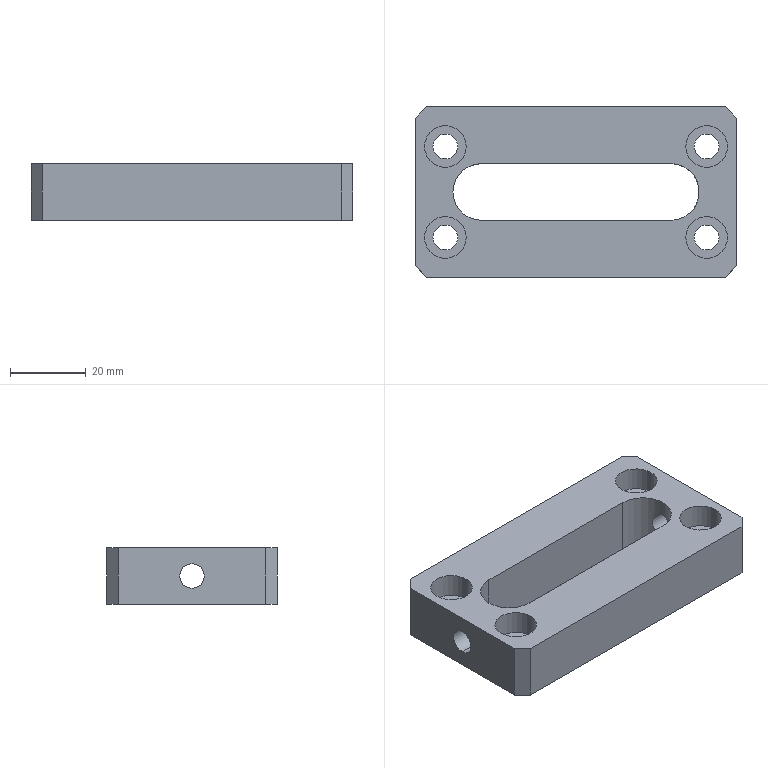Part | SolidWorks | features Chamfer 1, Extrusion 1, HoleWzd 1, ICE 1 | 1 solid | 39 faces | box 85 x 45 x 15 mm | volume 38919 mm3 | cylinder 23 | plane 16 | commonest cylinder face diameters 6.6 x8 11 x8 6.5 x4 15 x3
STEP:
#1=CARTESIAN_POINT('',(-32.5,0.,10.75));
#2=VERTEX_POINT('',#1);
#3=CARTESIAN_POINT('',(-32.5,0.,4.25));
#4=VERTEX_POINT('',#3);
#5=CARTESIAN_POINT('',(-32.5,0.,10.75));
#6=CARTESIAN_POINT('',(-32.5,-0.2176,10.75));
#7=CARTESIAN_POINT('',(-32.491,-0.4312,10.728));
#8=CARTESIAN_POINT('',(-32.455,-0.8504,10.644));
#9=CARTESIAN_POINT('',(-32.428,-1.058,10.58));
#10=CARTESIAN_POINT('',(-32.361,-1.451,10.416));
#11=CARTESIAN_POINT('',(-32.321,-1.637,10.316));
#12=CARTESIAN_POINT('',(-32.234,-1.988,10.08));
#13=CARTESIAN_POINT('',(-32.186,-2.152,9.944));
#14=CARTESIAN_POINT('',(-32.091,-2.448,9.648));
#15=CARTESIAN_POINT('',(-32.043,-2.582,9.485));
#16=CARTESIAN_POINT('',(-31.952,-2.818,9.133));
#17=CARTESIAN_POINT('',(-31.91,-2.917,8.948));
#18=CARTESIAN_POINT('',(-31.839,-3.08,8.558));
#19=CARTESIAN_POINT('',(-31.809,-3.144,8.351));
#20=CARTESIAN_POINT('',(-31.77,-3.229,7.93));
#21=CARTESIAN_POINT('',(-31.759,-3.25,7.717));
#22=CARTESIAN_POINT('',(-31.759,-3.25,7.287));
#23=CARTESIAN_POINT('',(-31.77,-3.228,7.069));
#24=CARTESIAN_POINT('',(-31.809,-3.144,6.65));
#25=CARTESIAN_POINT('',(-31.838,-3.081,6.445));
#26=CARTESIAN_POINT('',(-31.91,-2.916,6.05));
#27=CARTESIAN_POINT('',(-31.952,-2.816,5.864));
#28=CARTESIAN_POINT('',(-32.043,-2.581,5.514));
#29=CARTESIAN_POINT('',(-32.092,-2.446,5.349));
#30=CARTESIAN_POINT('',(-32.187,-2.149,5.053));
#31=CARTESIAN_POINT('',(-32.234,-1.987,4.92));
#32=CARTESIAN_POINT('',(-32.322,-1.636,4.684));
#33=CARTESIAN_POINT('',(-32.362,-1.447,4.582));
#34=CARTESIAN_POINT('',(-32.428,-1.057,4.419));
#35=CARTESIAN_POINT('',(-32.454,-0.8534,4.357));
#36=CARTESIAN_POINT('',(-32.491,-0.4282,4.271));
#37=CARTESIAN_POINT('',(-32.5,-0.2144,4.25));
#38=CARTESIAN_POINT('',(-32.5,0.,4.25));
#39=B_SPLINE_CURVE_WITH_KNOTS('',3,(#5,#6,#7,#8,#9,#10,#11,#12,#13,#14,#15,#16,#17,#18,#19,#20,#21,#22,#23,#24,#25,#26,#27,#28,#29,#30,#31,#32,#33,#34,#35,#36,#37,#38),.UNSPECIFIED.,.F.,.F.,(4,2,2,2,2,2,2,2,2,2,2,2,2,2,2,2,4),(0.,0.0006431,0.001286,0.001929,0.002573,0.003216,0.003859,0.004502,0.005145,0.005788,0.006431,0.007074,0.007718,0.008361,0.009004,0.009647,0.01029),.UNSPECIFIED.);
#40=EDGE_CURVE('',#2,#4,#39,.T.);
#41=ORIENTED_EDGE('',*,*,#40,.T.);
#42=CARTESIAN_POINT('',(-42.5,0.,4.25));
#43=VERTEX_POINT('',#42);
#44=CARTESIAN_POINT('',(119.5,0.,4.25));
#45=DIRECTION('',(-1.,0.,0.));
#46=VECTOR('',#45,1000.);
#47=LINE('',#44,#46);
#48=EDGE_CURVE('',#4,#43,#47,.T.);
#49=ORIENTED_EDGE('',*,*,#48,.T.);
#50=CARTESIAN_POINT('',(-42.5,0.,10.75));
#51=VERTEX_POINT('',#50);
#52=CARTESIAN_POINT('',(-42.5,0.,7.5));
#53=DIRECTION('',(-1.,0.,0.));
#54=DIRECTION('',(0.,0.,1.));
#55=AXIS2_PLACEMENT_3D('',#52,#53,#54);
#56=CIRCLE('',#55,3.25);
#57=EDGE_CURVE('',#43,#51,#56,.T.);
#58=ORIENTED_EDGE('',*,*,#57,.T.);
#59=CARTESIAN_POINT('',(119.5,0.,10.75));
#60=DIRECTION('',(-1.,0.,0.));
#61=VECTOR('',#60,1000.);
#62=LINE('',#59,#61);
#63=EDGE_CURVE('',#2,#51,#62,.T.);
#64=ORIENTED_EDGE('',*,*,#63,.F.);
#65=EDGE_LOOP('',(#41,#49,#58,#64));
#66=FACE_OUTER_BOUND('',#65,.T.);
#67=CARTESIAN_POINT('',(119.5,0.,7.5));
#68=DIRECTION('',(-1.,0.,0.));
#69=DIRECTION('',(0.,0.,1.));
#70=AXIS2_PLACEMENT_3D('',#67,#68,#69);
#71=CYLINDRICAL_SURFACE('',#70,3.25);
#72=ADVANCED_FACE('',(#66),#71,.F.);
#73=CARTESIAN_POINT('',(42.5,0.,4.25));
#74=VERTEX_POINT('',#73);
#75=CARTESIAN_POINT('',(42.5,0.,10.75));
#76=VERTEX_POINT('',#75);
#77=CARTESIAN_POINT('',(42.5,0.,7.5));
#78=DIRECTION('',(-1.,0.,0.));
#79=DIRECTION('',(0.,0.,1.));
#80=AXIS2_PLACEMENT_3D('',#77,#78,#79);
#81=CIRCLE('',#80,3.25);
#82=EDGE_CURVE('',#74,#76,#81,.T.);
#83=ORIENTED_EDGE('',*,*,#82,.F.);
#84=CARTESIAN_POINT('',(32.5,0.,4.25));
#85=VERTEX_POINT('',#84);
#86=CARTESIAN_POINT('',(119.5,0.,4.25));
#87=DIRECTION('',(-1.,0.,0.));
#88=VECTOR('',#87,1000.);
#89=LINE('',#86,#88);
#90=EDGE_CURVE('',#74,#85,#89,.T.);
#91=ORIENTED_EDGE('',*,*,#90,.T.);
#92=CARTESIAN_POINT('',(32.5,0.,10.75));
#93=VERTEX_POINT('',#92);
#94=CARTESIAN_POINT('',(32.5,0.,4.25));
#95=CARTESIAN_POINT('',(32.5,-0.2142,4.25));
#96=CARTESIAN_POINT('',(32.491,-0.4319,4.272));
#97=CARTESIAN_POINT('',(32.454,-0.8529,4.357));
#98=CARTESIAN_POINT('',(32.428,-1.056,4.419));
#99=CARTESIAN_POINT('',(32.361,-1.45,4.584));
#100=CARTESIAN_POINT('',(32.321,-1.639,4.686));
#101=CARTESIAN_POINT('',(32.234,-1.988,4.92));
#102=CARTESIAN_POINT('',(32.187,-2.151,5.055));
#103=CARTESIAN_POINT('',(32.091,-2.449,5.353));
#104=CARTESIAN_POINT('',(32.043,-2.582,5.515));
#105=CARTESIAN_POINT('',(31.952,-2.816,5.864));
#106=CARTESIAN_POINT('',(31.91,-2.918,6.053));
#107=CARTESIAN_POINT('',(31.839,-3.081,6.444));
#108=CARTESIAN_POINT('',(31.81,-3.143,6.646));
#109=CARTESIAN_POINT('',(31.77,-3.228,7.066));
#110=CARTESIAN_POINT('',(31.759,-3.25,7.284));
#111=CARTESIAN_POINT('',(31.759,-3.25,7.713));
#112=CARTESIAN_POINT('',(31.769,-3.229,7.927));
#113=CARTESIAN_POINT('',(31.809,-3.144,8.351));
#114=CARTESIAN_POINT('',(31.838,-3.081,8.555));
#115=CARTESIAN_POINT('',(31.91,-2.918,8.947));
#116=CARTESIAN_POINT('',(31.952,-2.816,9.136));
#117=CARTESIAN_POINT('',(32.043,-2.582,9.485));
#118=CARTESIAN_POINT('',(32.091,-2.449,9.647));
#119=CARTESIAN_POINT('',(32.235,-2.001,10.095));
#120=CARTESIAN_POINT('',(32.327,-1.649,10.333));
#121=CARTESIAN_POINT('',(32.428,-1.056,10.581));
#122=CARTESIAN_POINT('',(32.454,-0.853,10.643));
#123=CARTESIAN_POINT('',(32.49,-0.4346,10.728));
#124=CARTESIAN_POINT('',(32.5,-0.2174,10.75));
#125=CARTESIAN_POINT('',(32.5,0.,10.75));
#126=B_SPLINE_CURVE_WITH_KNOTS('',3,(#94,#95,#96,#97,#98,#99,#100,#101,#102,#103,#104,#105,#106,#107,#108,#109,#110,#111,#112,#113,#114,#115,#116,#117,#118,#119,#120,#121,#122,#123,#124,#125),.UNSPECIFIED.,.F.,.F.,(4,2,2,2,2,2,2,2,2,2,2,2,2,2,2,4),(0.01029,0.01093,0.01158,0.01222,0.01286,0.0135,0.01415,0.01479,0.01543,0.01607,0.01672,0.01736,0.018,0.01929,0.01993,0.02057),.UNSPECIFIED.);
#127=EDGE_CURVE('',#85,#93,#126,.T.);
#128=ORIENTED_EDGE('',*,*,#127,.T.);
#129=CARTESIAN_POINT('',(119.5,0.,10.75));
#130=DIRECTION('',(-1.,0.,0.));
#131=VECTOR('',#130,1000.);
#132=LINE('',#129,#131);
#133=EDGE_CURVE('',#76,#93,#132,.T.);
#134=ORIENTED_EDGE('',*,*,#133,.F.);
#135=EDGE_LOOP('',(#83,#91,#128,#134));
#136=FACE_OUTER_BOUND('',#135,.T.);
#137=CARTESIAN_POINT('',(119.5,0.,7.5));
#138=DIRECTION('',(-1.,0.,0.));
#139=DIRECTION('',(0.,0.,1.));
#140=AXIS2_PLACEMENT_3D('',#137,#138,#139);
#141=CYLINDRICAL_SURFACE('',#140,3.25);
#142=ADVANCED_FACE('',(#136),#141,.F.);
#143=CARTESIAN_POINT('',(-40.,12.,8.6));
#144=VERTEX_POINT('',#143);
#145=CARTESIAN_POINT('',(-29.,12.,8.6));
#146=VERTEX_POINT('',#145);
#147=CARTESIAN_POINT('',(-34.5,12.,8.6));
#148=DIRECTION('',(0.,0.,1.));
#149=DIRECTION('',(1.,0.,0.));
#150=AXIS2_PLACEMENT_3D('',#147,#148,#149);
#151=CIRCLE('',#150,5.5);
#152=EDGE_CURVE('',#144,#146,#151,.T.);
#153=ORIENTED_EDGE('',*,*,#152,.F.);
#154=CARTESIAN_POINT('',(-40.,12.,15.));
#155=VERTEX_POINT('',#154);
#156=CARTESIAN_POINT('',(-40.,12.,15.));
#157=DIRECTION('',(0.,0.,1.));
#158=VECTOR('',#157,1000.);
#159=LINE('',#156,#158);
#160=EDGE_CURVE('',#144,#155,#159,.T.);
#161=ORIENTED_EDGE('',*,*,#160,.T.);
#162=CARTESIAN_POINT('',(-29.,12.,15.));
#163=VERTEX_POINT('',#162);
#164=CARTESIAN_POINT('',(-34.5,12.,15.));
#165=DIRECTION('',(0.,0.,1.));
#166=DIRECTION('',(1.,0.,0.));
#167=AXIS2_PLACEMENT_3D('',#164,#165,#166);
#168=CIRCLE('',#167,5.5);
#169=EDGE_CURVE('',#155,#163,#168,.T.);
#170=ORIENTED_EDGE('',*,*,#169,.T.);
#171=CARTESIAN_POINT('',(-29.,12.,15.));
#172=DIRECTION('',(0.,0.,1.));
#173=VECTOR('',#172,1000.);
#174=LINE('',#171,#173);
#175=EDGE_CURVE('',#146,#163,#174,.T.);
#176=ORIENTED_EDGE('',*,*,#175,.F.);
#177=EDGE_LOOP('',(#153,#161,#170,#176));
#178=FACE_OUTER_BOUND('',#177,.T.);
#179=CARTESIAN_POINT('',(-34.5,12.,15.));
#180=DIRECTION('',(0.,0.,1.));
#181=DIRECTION('',(1.,0.,0.));
#182=AXIS2_PLACEMENT_3D('',#179,#180,#181);
#183=CYLINDRICAL_SURFACE('',#182,5.5);
#184=ADVANCED_FACE('',(#178),#183,.F.);
#185=CARTESIAN_POINT('',(-37.8,12.,0.));
#186=VERTEX_POINT('',#185);
#187=CARTESIAN_POINT('',(-31.2,12.,0.));
#188=VERTEX_POINT('',#187);
#189=CARTESIAN_POINT('',(-34.5,12.,0.));
#190=DIRECTION('',(0.,0.,1.));
#191=DIRECTION('',(1.,0.,0.));
#192=AXIS2_PLACEMENT_3D('',#189,#190,#191);
#193=CIRCLE('',#192,3.3);
#194=EDGE_CURVE('',#186,#188,#193,.T.);
#195=ORIENTED_EDGE('',*,*,#194,.F.);
#196=CARTESIAN_POINT('',(-37.8,12.,8.6));
#197=VERTEX_POINT('',#196);
#198=CARTESIAN_POINT('',(-37.8,12.,15.));
#199=DIRECTION('',(0.,0.,1.));
#200=VECTOR('',#199,1000.);
#201=LINE('',#198,#200);
#202=EDGE_CURVE('',#186,#197,#201,.T.);
#203=ORIENTED_EDGE('',*,*,#202,.T.);
#204=CARTESIAN_POINT('',(-31.2,12.,8.6));
#205=VERTEX_POINT('',#204);
#206=CARTESIAN_POINT('',(-34.5,12.,8.6));
#207=DIRECTION('',(0.,0.,1.));
#208=DIRECTION('',(1.,0.,0.));
#209=AXIS2_PLACEMENT_3D('',#206,#207,#208);
#210=CIRCLE('',#209,3.3);
#211=EDGE_CURVE('',#197,#205,#210,.T.);
#212=ORIENTED_EDGE('',*,*,#211,.T.);
#213=CARTESIAN_POINT('',(-31.2,12.,15.));
#214=DIRECTION('',(0.,0.,1.));
#215=VECTOR('',#214,1000.);
#216=LINE('',#213,#215);
#217=EDGE_CURVE('',#188,#205,#216,.T.);
#218=ORIENTED_EDGE('',*,*,#217,.F.);
#219=EDGE_LOOP('',(#195,#203,#212,#218));
#220=FACE_OUTER_BOUND('',#219,.T.);
#221=CARTESIAN_POINT('',(-34.5,12.,15.));
#222=DIRECTION('',(0.,0.,1.));
#223=DIRECTION('',(1.,0.,0.));
#224=AXIS2_PLACEMENT_3D('',#221,#222,#223);
#225=CYLINDRICAL_SURFACE('',#224,3.3);
#226=ADVANCED_FACE('',(#220),#225,.F.);
#227=CARTESIAN_POINT('',(-40.,-12.,8.6));
#228=VERTEX_POINT('',#227);
#229=CARTESIAN_POINT('',(-29.,-12.,8.6));
#230=VERTEX_POINT('',#229);
#231=CARTESIAN_POINT('',(-34.5,-12.,8.6));
#232=DIRECTION('',(0.,0.,1.));
#233=DIRECTION('',(1.,0.,0.));
#234=AXIS2_PLACEMENT_3D('',#231,#232,#233);
#235=CIRCLE('',#234,5.5);
#236=EDGE_CURVE('',#228,#230,#235,.T.);
#237=ORIENTED_EDGE('',*,*,#236,.F.);
#238=CARTESIAN_POINT('',(-40.,-12.,15.));
#239=VERTEX_POINT('',#238);
#240=CARTESIAN_POINT('',(-40.,-12.,15.));
#241=DIRECTION('',(0.,0.,1.));
#242=VECTOR('',#241,1000.);
#243=LINE('',#240,#242);
#244=EDGE_CURVE('',#228,#239,#243,.T.);
#245=ORIENTED_EDGE('',*,*,#244,.T.);
#246=CARTESIAN_POINT('',(-29.,-12.,15.));
#247=VERTEX_POINT('',#246);
#248=CARTESIAN_POINT('',(-34.5,-12.,15.));
#249=DIRECTION('',(0.,0.,1.));
#250=DIRECTION('',(1.,0.,0.));
#251=AXIS2_PLACEMENT_3D('',#248,#249,#250);
#252=CIRCLE('',#251,5.5);
#253=EDGE_CURVE('',#239,#247,#252,.T.);
#254=ORIENTED_EDGE('',*,*,#253,.T.);
#255=CARTESIAN_POINT('',(-29.,-12.,15.));
#256=DIRECTION('',(0.,0.,1.));
#257=VECTOR('',#256,1000.);
#258=LINE('',#255,#257);
#259=EDGE_CURVE('',#230,#247,#258,.T.);
#260=ORIENTED_EDGE('',*,*,#259,.F.);
#261=EDGE_LOOP('',(#237,#245,#254,#260));
#262=FACE_OUTER_BOUND('',#261,.T.);
#263=CARTESIAN_POINT('',(-34.5,-12.,15.));
#264=DIRECTION('',(0.,0.,1.));
#265=DIRECTION('',(1.,0.,0.));
#266=AXIS2_PLACEMENT_3D('',#263,#264,#265);
#267=CYLINDRICAL_SURFACE('',#266,5.5);
#268=ADVANCED_FACE('',(#262),#267,.F.);
#269=CARTESIAN_POINT('',(-37.8,-12.,0.));
#270=VERTEX_POINT('',#269);
#271=CARTESIAN_POINT('',(-31.2,-12.,0.));
#272=VERTEX_POINT('',#271);
#273=CARTESIAN_POINT('',(-34.5,-12.,0.));
#274=DIRECTION('',(0.,0.,1.));
#275=DIRECTION('',(1.,0.,0.));
#276=AXIS2_PLACEMENT_3D('',#273,#274,#275);
#277=CIRCLE('',#276,3.3);
#278=EDGE_CURVE('',#270,#272,#277,.T.);
#279=ORIENTED_EDGE('',*,*,#278,.F.);
#280=CARTESIAN_POINT('',(-37.8,-12.,8.6));
#281=VERTEX_POINT('',#280);
#282=CARTESIAN_POINT('',(-37.8,-12.,15.));
#283=DIRECTION('',(0.,0.,1.));
#284=VECTOR('',#283,1000.);
#285=LINE('',#282,#284);
#286=EDGE_CURVE('',#270,#281,#285,.T.);
#287=ORIENTED_EDGE('',*,*,#286,.T.);
#288=CARTESIAN_POINT('',(-31.2,-12.,8.6));
#289=VERTEX_POINT('',#288);
#290=CARTESIAN_POINT('',(-34.5,-12.,8.6));
#291=DIRECTION('',(0.,0.,1.));
#292=DIRECTION('',(1.,0.,0.));
#293=AXIS2_PLACEMENT_3D('',#290,#291,#292);
#294=CIRCLE('',#293,3.3);
#295=EDGE_CURVE('',#281,#289,#294,.T.);
#296=ORIENTED_EDGE('',*,*,#295,.T.);
#297=CARTESIAN_POINT('',(-31.2,-12.,15.));
#298=DIRECTION('',(0.,0.,1.));
#299=VECTOR('',#298,1000.);
#300=LINE('',#297,#299);
#301=EDGE_CURVE('',#272,#289,#300,.T.);
#302=ORIENTED_EDGE('',*,*,#301,.F.);
#303=EDGE_LOOP('',(#279,#287,#296,#302));
#304=FACE_OUTER_BOUND('',#303,.T.);
#305=CARTESIAN_POINT('',(-34.5,-12.,15.));
#306=DIRECTION('',(0.,0.,1.));
#307=DIRECTION('',(1.,0.,0.));
#308=AXIS2_PLACEMENT_3D('',#305,#306,#307);
#309=CYLINDRICAL_SURFACE('',#308,3.3);
#310=ADVANCED_FACE('',(#304),#309,.F.);
#311=CARTESIAN_POINT('',(29.,-12.,8.6));
#312=VERTEX_POINT('',#311);
#313=CARTESIAN_POINT('',(40.,-12.,8.6));
#314=VERTEX_POINT('',#313);
#315=CARTESIAN_POINT('',(34.5,-12.,8.6));
#316=DIRECTION('',(0.,0.,1.));
#317=DIRECTION('',(1.,0.,0.));
#318=AXIS2_PLACEMENT_3D('',#315,#316,#317);
#319=CIRCLE('',#318,5.5);
#320=EDGE_CURVE('',#312,#314,#319,.T.);
#321=ORIENTED_EDGE('',*,*,#320,.F.);
#322=CARTESIAN_POINT('',(29.,-12.,15.));
#323=VERTEX_POINT('',#322);
#324=CARTESIAN_POINT('',(29.,-12.,15.));
#325=DIRECTION('',(0.,0.,1.));
#326=VECTOR('',#325,1000.);
#327=LINE('',#324,#326);
#328=EDGE_CURVE('',#312,#323,#327,.T.);
#329=ORIENTED_EDGE('',*,*,#328,.T.);
#330=CARTESIAN_POINT('',(40.,-12.,15.));
#331=VERTEX_POINT('',#330);
#332=CARTESIAN_POINT('',(34.5,-12.,15.));
#333=DIRECTION('',(0.,0.,1.));
#334=DIRECTION('',(1.,0.,0.));
#335=AXIS2_PLACEMENT_3D('',#332,#333,#334);
#336=CIRCLE('',#335,5.5);
#337=EDGE_CURVE('',#323,#331,#336,.T.);
#338=ORIENTED_EDGE('',*,*,#337,.T.);
#339=CARTESIAN_POINT('',(40.,-12.,15.));
#340=DIRECTION('',(0.,0.,1.));
#341=VECTOR('',#340,1000.);
#342=LINE('',#339,#341);
#343=EDGE_CURVE('',#314,#331,#342,.T.);
#344=ORIENTED_EDGE('',*,*,#343,.F.);
#345=EDGE_LOOP('',(#321,#329,#338,#344));
#346=FACE_OUTER_BOUND('',#345,.T.);
#347=CARTESIAN_POINT('',(34.5,-12.,15.));
#348=DIRECTION('',(0.,0.,1.));
#349=DIRECTION('',(1.,0.,0.));
#350=AXIS2_PLACEMENT_3D('',#347,#348,#349);
#351=CYLINDRICAL_SURFACE('',#350,5.5);
#352=ADVANCED_FACE('',(#346),#351,.F.);
#353=CARTESIAN_POINT('',(31.2,-12.,0.));
#354=VERTEX_POINT('',#353);
#355=CARTESIAN_POINT('',(37.8,-12.,0.));
#356=VERTEX_POINT('',#355);
#357=CARTESIAN_POINT('',(34.5,-12.,0.));
#358=DIRECTION('',(0.,0.,1.));
#359=DIRECTION('',(1.,0.,0.));
#360=AXIS2_PLACEMENT_3D('',#357,#358,#359);
#361=CIRCLE('',#360,3.3);
#362=EDGE_CURVE('',#354,#356,#361,.T.);
#363=ORIENTED_EDGE('',*,*,#362,.F.);
#364=CARTESIAN_POINT('',(31.2,-12.,8.6));
#365=VERTEX_POINT('',#364);
#366=CARTESIAN_POINT('',(31.2,-12.,15.));
#367=DIRECTION('',(0.,0.,1.));
#368=VECTOR('',#367,1000.);
#369=LINE('',#366,#368);
#370=EDGE_CURVE('',#354,#365,#369,.T.);
#371=ORIENTED_EDGE('',*,*,#370,.T.);
#372=CARTESIAN_POINT('',(37.8,-12.,8.6));
#373=VERTEX_POINT('',#372);
#374=CARTESIAN_POINT('',(34.5,-12.,8.6));
#375=DIRECTION('',(0.,0.,1.));
#376=DIRECTION('',(1.,0.,0.));
#377=AXIS2_PLACEMENT_3D('',#374,#375,#376);
#378=CIRCLE('',#377,3.3);
#379=EDGE_CURVE('',#365,#373,#378,.T.);
#380=ORIENTED_EDGE('',*,*,#379,.T.);
#381=CARTESIAN_POINT('',(37.8,-12.,15.));
#382=DIRECTION('',(0.,0.,1.));
#383=VECTOR('',#382,1000.);
#384=LINE('',#381,#383);
#385=EDGE_CURVE('',#356,#373,#384,.T.);
#386=ORIENTED_EDGE('',*,*,#385,.F.);
#387=EDGE_LOOP('',(#363,#371,#380,#386));
#388=FACE_OUTER_BOUND('',#387,.T.);
#389=CARTESIAN_POINT('',(34.5,-12.,15.));
#390=DIRECTION('',(0.,0.,1.));
#391=DIRECTION('',(1.,0.,0.));
#392=AXIS2_PLACEMENT_3D('',#389,#390,#391);
#393=CYLINDRICAL_SURFACE('',#392,3.3);
#394=ADVANCED_FACE('',(#388),#393,.F.);
#395=CARTESIAN_POINT('',(29.,12.,8.6));
#396=VERTEX_POINT('',#395);
#397=CARTESIAN_POINT('',(40.,12.,8.6));
#398=VERTEX_POINT('',#397);
#399=CARTESIAN_POINT('',(34.5,12.,8.6));
#400=DIRECTION('',(0.,0.,1.));
#401=DIRECTION('',(1.,0.,0.));
#402=AXIS2_PLACEMENT_3D('',#399,#400,#401);
#403=CIRCLE('',#402,5.5);
#404=EDGE_CURVE('',#396,#398,#403,.T.);
#405=ORIENTED_EDGE('',*,*,#404,.F.);
#406=CARTESIAN_POINT('',(29.,12.,15.));
#407=VERTEX_POINT('',#406);
#408=CARTESIAN_POINT('',(29.,12.,15.));
#409=DIRECTION('',(0.,0.,1.));
#410=VECTOR('',#409,1000.);
#411=LINE('',#408,#410);
#412=EDGE_CURVE('',#396,#407,#411,.T.);
#413=ORIENTED_EDGE('',*,*,#412,.T.);
#414=CARTESIAN_POINT('',(40.,12.,15.));
#415=VERTEX_POINT('',#414);
#416=CARTESIAN_POINT('',(34.5,12.,15.));
#417=DIRECTION('',(0.,0.,1.));
#418=DIRECTION('',(1.,0.,0.));
#419=AXIS2_PLACEMENT_3D('',#416,#417,#418);
#420=CIRCLE('',#419,5.5);
#421=EDGE_CURVE('',#407,#415,#420,.T.);
#422=ORIENTED_EDGE('',*,*,#421,.T.);
#423=CARTESIAN_POINT('',(40.,12.,15.));
#424=DIRECTION('',(0.,0.,1.));
#425=VECTOR('',#424,1000.);
#426=LINE('',#423,#425);
#427=EDGE_CURVE('',#398,#415,#426,.T.);
#428=ORIENTED_EDGE('',*,*,#427,.F.);
#429=EDGE_LOOP('',(#405,#413,#422,#428));
#430=FACE_OUTER_BOUND('',#429,.T.);
#431=CARTESIAN_POINT('',(34.5,12.,15.));
#432=DIRECTION('',(0.,0.,1.));
#433=DIRECTION('',(1.,0.,0.));
#434=AXIS2_PLACEMENT_3D('',#431,#432,#433);
#435=CYLINDRICAL_SURFACE('',#434,5.5);
#436=ADVANCED_FACE('',(#430),#435,.F.);
#437=CARTESIAN_POINT('',(31.2,12.,0.));
#438=VERTEX_POINT('',#437);
#439=CARTESIAN_POINT('',(37.8,12.,0.));
#440=VERTEX_POINT('',#439);
#441=CARTESIAN_POINT('',(34.5,12.,0.));
#442=DIRECTION('',(0.,0.,1.));
#443=DIRECTION('',(1.,0.,0.));
#444=AXIS2_PLACEMENT_3D('',#441,#442,#443);
#445=CIRCLE('',#444,3.3);
#446=EDGE_CURVE('',#438,#440,#445,.T.);
#447=ORIENTED_EDGE('',*,*,#446,.F.);
#448=CARTESIAN_POINT('',(31.2,12.,8.6));
#449=VERTEX_POINT('',#448);
#450=CARTESIAN_POINT('',(31.2,12.,15.));
#451=DIRECTION('',(0.,0.,1.));
#452=VECTOR('',#451,1000.);
#453=LINE('',#450,#452);
#454=EDGE_CURVE('',#438,#449,#453,.T.);
#455=ORIENTED_EDGE('',*,*,#454,.T.);
#456=CARTESIAN_POINT('',(37.8,12.,8.6));
#457=VERTEX_POINT('',#456);
#458=CARTESIAN_POINT('',(34.5,12.,8.6));
#459=DIRECTION('',(0.,0.,1.));
#460=DIRECTION('',(1.,0.,0.));
#461=AXIS2_PLACEMENT_3D('',#458,#459,#460);
#462=CIRCLE('',#461,3.3);
#463=EDGE_CURVE('',#449,#457,#462,.T.);
#464=ORIENTED_EDGE('',*,*,#463,.T.);
#465=CARTESIAN_POINT('',(37.8,12.,15.));
#466=DIRECTION('',(0.,0.,1.));
#467=VECTOR('',#466,1000.);
#468=LINE('',#465,#467);
#469=EDGE_CURVE('',#440,#457,#468,.T.);
#470=ORIENTED_EDGE('',*,*,#469,.F.);
#471=EDGE_LOOP('',(#447,#455,#464,#470));
#472=FACE_OUTER_BOUND('',#471,.T.);
#473=CARTESIAN_POINT('',(34.5,12.,15.));
#474=DIRECTION('',(0.,0.,1.));
#475=DIRECTION('',(1.,0.,0.));
#476=AXIS2_PLACEMENT_3D('',#473,#474,#475);
#477=CYLINDRICAL_SURFACE('',#476,3.3);
#478=ADVANCED_FACE('',(#472),#477,.F.);
#479=CARTESIAN_POINT('',(-25.,7.5,15.));
#480=VERTEX_POINT('',#479);
#481=CARTESIAN_POINT('',(-32.5,0.,15.));
#482=VERTEX_POINT('',#481);
#483=CARTESIAN_POINT('',(-25.,0.,15.));
#484=DIRECTION('',(0.,0.,1.));
#485=DIRECTION('',(1.,0.,0.));
#486=AXIS2_PLACEMENT_3D('',#483,#484,#485);
#487=CIRCLE('',#486,7.5);
#488=EDGE_CURVE('',#480,#482,#487,.T.);
#489=ORIENTED_EDGE('',*,*,#488,.T.);
#490=CARTESIAN_POINT('',(-32.5,0.,15.));
#491=DIRECTION('',(0.,0.,-1.));
#492=VECTOR('',#491,1000.);
#493=LINE('',#490,#492);
#494=EDGE_CURVE('',#482,#2,#493,.T.);
#495=ORIENTED_EDGE('',*,*,#494,.T.);
#496=CARTESIAN_POINT('',(-32.5,0.,4.25));
#497=CARTESIAN_POINT('',(-32.5,0.2142,4.25));
#498=CARTESIAN_POINT('',(-32.491,0.4319,4.272));
#499=CARTESIAN_POINT('',(-32.454,0.8529,4.357));
#500=CARTESIAN_POINT('',(-32.428,1.056,4.419));
#501=CARTESIAN_POINT('',(-32.361,1.45,4.584));
#502=CARTESIAN_POINT('',(-32.321,1.639,4.686));
#503=CARTESIAN_POINT('',(-32.234,1.988,4.92));
#504=CARTESIAN_POINT('',(-32.187,2.151,5.055));
#505=CARTESIAN_POINT('',(-32.091,2.449,5.353));
#506=CARTESIAN_POINT('',(-32.043,2.582,5.515));
#507=CARTESIAN_POINT('',(-31.952,2.816,5.864));
#508=CARTESIAN_POINT('',(-31.91,2.918,6.053));
#509=CARTESIAN_POINT('',(-31.839,3.081,6.444));
#510=CARTESIAN_POINT('',(-31.81,3.143,6.646));
#511=CARTESIAN_POINT('',(-31.77,3.228,7.066));
#512=CARTESIAN_POINT('',(-31.759,3.25,7.284));
#513=CARTESIAN_POINT('',(-31.759,3.25,7.713));
#514=CARTESIAN_POINT('',(-31.769,3.229,7.927));
#515=CARTESIAN_POINT('',(-31.809,3.144,8.351));
#516=CARTESIAN_POINT('',(-31.838,3.081,8.555));
#517=CARTESIAN_POINT('',(-31.91,2.918,8.947));
#518=CARTESIAN_POINT('',(-31.952,2.816,9.136));
#519=CARTESIAN_POINT('',(-32.043,2.582,9.485));
#520=CARTESIAN_POINT('',(-32.091,2.449,9.647));
#521=CARTESIAN_POINT('',(-32.235,2.001,10.095));
#522=CARTESIAN_POINT('',(-32.327,1.649,10.333));
#523=CARTESIAN_POINT('',(-32.428,1.056,10.581));
#524=CARTESIAN_POINT('',(-32.454,0.853,10.643));
#525=CARTESIAN_POINT('',(-32.49,0.4346,10.728));
#526=CARTESIAN_POINT('',(-32.5,0.2174,10.75));
#527=CARTESIAN_POINT('',(-32.5,0.,10.75));
#528=B_SPLINE_CURVE_WITH_KNOTS('',3,(#496,#497,#498,#499,#500,#501,#502,#503,#504,#505,#506,#507,#508,#509,#510,#511,#512,#513,#514,#515,#516,#517,#518,#519,#520,#521,#522,#523,#524,#525,#526,#527),.UNSPECIFIED.,.F.,.F.,(4,2,2,2,2,2,2,2,2,2,2,2,2,2,2,4),(0.01029,0.01093,0.01158,0.01222,0.01286,0.0135,0.01415,0.01479,0.01543,0.01607,0.01672,0.01736,0.018,0.01929,0.01993,0.02057),.UNSPECIFIED.);
#529=EDGE_CURVE('',#4,#2,#528,.T.);
#530=ORIENTED_EDGE('',*,*,#529,.F.);
#531=CARTESIAN_POINT('',(-32.5,0.,0.));
#532=VERTEX_POINT('',#531);
#533=CARTESIAN_POINT('',(-32.5,0.,15.));
#534=DIRECTION('',(0.,0.,-1.));
#535=VECTOR('',#534,1000.);
#536=LINE('',#533,#535);
#537=EDGE_CURVE('',#4,#532,#536,.T.);
#538=ORIENTED_EDGE('',*,*,#537,.T.);
#539=CARTESIAN_POINT('',(-25.,7.5,0.));
#540=VERTEX_POINT('',#539);
#541=CARTESIAN_POINT('',(-25.,0.,0.));
#542=DIRECTION('',(0.,0.,1.));
#543=DIRECTION('',(1.,0.,0.));
#544=AXIS2_PLACEMENT_3D('',#541,#542,#543);
#545=CIRCLE('',#544,7.5);
#546=EDGE_CURVE('',#540,#532,#545,.T.);
#547=ORIENTED_EDGE('',*,*,#546,.F.);
#548=CARTESIAN_POINT('',(-25.,7.5,15.));
#549=DIRECTION('',(0.,0.,-1.));
#550=VECTOR('',#549,1000.);
#551=LINE('',#548,#550);
#552=EDGE_CURVE('',#480,#540,#551,.T.);
#553=ORIENTED_EDGE('',*,*,#552,.F.);
#554=EDGE_LOOP('',(#489,#495,#530,#538,#547,#553));
#555=FACE_OUTER_BOUND('',#554,.T.);
#556=CARTESIAN_POINT('',(-25.,0.,15.));
#557=DIRECTION('',(0.,0.,-1.));
#558=DIRECTION('',(-1.,0.,0.));
#559=AXIS2_PLACEMENT_3D('',#556,#557,#558);
#560=CYLINDRICAL_SURFACE('',#559,7.5);
#561=ADVANCED_FACE('',(#555),#560,.F.);
#562=CARTESIAN_POINT('',(-34.5,12.,15.));
#563=DIRECTION('',(0.,0.,1.));
#564=DIRECTION('',(1.,0.,0.));
#565=AXIS2_PLACEMENT_3D('',#562,#563,#564);
#566=CIRCLE('',#565,5.5);
#567=EDGE_CURVE('',#163,#155,#566,.T.);
#568=ORIENTED_EDGE('',*,*,#567,.F.);
#569=ORIENTED_EDGE('',*,*,#169,.F.);
#570=EDGE_LOOP('',(#568,#569));
#571=FACE_BOUND('',#570,.T.);
#572=CARTESIAN_POINT('',(-34.5,-12.,15.));
#573=DIRECTION('',(0.,0.,1.));
#574=DIRECTION('',(1.,0.,0.));
#575=AXIS2_PLACEMENT_3D('',#572,#573,#574);
#576=CIRCLE('',#575,5.5);
#577=EDGE_CURVE('',#247,#239,#576,.T.);
#578=ORIENTED_EDGE('',*,*,#577,.F.);
#579=ORIENTED_EDGE('',*,*,#253,.F.);
#580=EDGE_LOOP('',(#578,#579));
#581=FACE_BOUND('',#580,.T.);
#582=CARTESIAN_POINT('',(34.5,-12.,15.));
#583=DIRECTION('',(0.,0.,1.));
#584=DIRECTION('',(1.,0.,0.));
#585=AXIS2_PLACEMENT_3D('',#582,#583,#584);
#586=CIRCLE('',#585,5.5);
#587=EDGE_CURVE('',#331,#323,#586,.T.);
#588=ORIENTED_EDGE('',*,*,#587,.F.);
#589=ORIENTED_EDGE('',*,*,#337,.F.);
#590=EDGE_LOOP('',(#588,#589));
#591=FACE_BOUND('',#590,.T.);
#592=CARTESIAN_POINT('',(34.5,12.,15.));
#593=DIRECTION('',(0.,0.,1.));
#594=DIRECTION('',(1.,0.,0.));
#595=AXIS2_PLACEMENT_3D('',#592,#593,#594);
#596=CIRCLE('',#595,5.5);
#597=EDGE_CURVE('',#415,#407,#596,.T.);
#598=ORIENTED_EDGE('',*,*,#597,.F.);
#599=ORIENTED_EDGE('',*,*,#421,.F.);
#600=EDGE_LOOP('',(#598,#599));
#601=FACE_BOUND('',#600,.T.);
#602=CARTESIAN_POINT('',(-39.5,-22.5,15.));
#603=VERTEX_POINT('',#602);
#604=CARTESIAN_POINT('',(39.5,-22.5,15.));
#605=VERTEX_POINT('',#604);
#606=CARTESIAN_POINT('',(-42.5,-22.5,15.));
#607=DIRECTION('',(1.,0.,0.));
#608=VECTOR('',#607,1000.);
#609=LINE('',#606,#608);
#610=EDGE_CURVE('',#603,#605,#609,.T.);
#611=ORIENTED_EDGE('',*,*,#610,.T.);
#612=CARTESIAN_POINT('',(42.5,-19.5,15.));
#613=VERTEX_POINT('',#612);
#614=CARTESIAN_POINT('',(42.5,-19.5,15.));
#615=DIRECTION('',(0.7071,0.7071,0.));
#616=VECTOR('',#615,1000.);
#617=LINE('',#614,#616);
#618=EDGE_CURVE('',#605,#613,#617,.T.);
#619=ORIENTED_EDGE('',*,*,#618,.T.);
#620=CARTESIAN_POINT('',(42.5,19.5,15.));
#621=VERTEX_POINT('',#620);
#622=CARTESIAN_POINT('',(42.5,-22.5,15.));
#623=DIRECTION('',(0.,1.,0.));
#624=VECTOR('',#623,1000.);
#625=LINE('',#622,#624);
#626=EDGE_CURVE('',#613,#621,#625,.T.);
#627=ORIENTED_EDGE('',*,*,#626,.T.);
#628=CARTESIAN_POINT('',(39.5,22.5,15.));
#629=VERTEX_POINT('',#628);
#630=CARTESIAN_POINT('',(39.5,22.5,15.));
#631=DIRECTION('',(-0.7071,0.7071,0.));
#632=VECTOR('',#631,1000.);
#633=LINE('',#630,#632);
#634=EDGE_CURVE('',#621,#629,#633,.T.);
#635=ORIENTED_EDGE('',*,*,#634,.T.);
#636=CARTESIAN_POINT('',(-39.5,22.5,15.));
#637=VERTEX_POINT('',#636);
#638=CARTESIAN_POINT('',(-42.5,22.5,15.));
#639=DIRECTION('',(-1.,0.,0.));
#640=VECTOR('',#639,1000.);
#641=LINE('',#638,#640);
#642=EDGE_CURVE('',#629,#637,#641,.T.);
#643=ORIENTED_EDGE('',*,*,#642,.T.);
#644=CARTESIAN_POINT('',(-42.5,19.5,15.));
#645=VERTEX_POINT('',#644);
#646=CARTESIAN_POINT('',(-42.5,19.5,15.));
#647=DIRECTION('',(-0.7071,-0.7071,0.));
#648=VECTOR('',#647,1000.);
#649=LINE('',#646,#648);
#650=EDGE_CURVE('',#637,#645,#649,.T.);
#651=ORIENTED_EDGE('',*,*,#650,.T.);
#652=CARTESIAN_POINT('',(-42.5,-19.5,15.));
#653=VERTEX_POINT('',#652);
#654=CARTESIAN_POINT('',(-42.5,-22.5,15.));
#655=DIRECTION('',(0.,-1.,0.));
#656=VECTOR('',#655,1000.);
#657=LINE('',#654,#656);
#658=EDGE_CURVE('',#645,#653,#657,.T.);
#659=ORIENTED_EDGE('',*,*,#658,.T.);
#660=CARTESIAN_POINT('',(-39.5,-22.5,15.));
#661=DIRECTION('',(0.7071,-0.7071,0.));
#662=VECTOR('',#661,1000.);
#663=LINE('',#660,#662);
#664=EDGE_CURVE('',#653,#603,#663,.T.);
#665=ORIENTED_EDGE('',*,*,#664,.T.);
#666=EDGE_LOOP('',(#611,#619,#627,#635,#643,#651,#659,#665));
#667=FACE_OUTER_BOUND('',#666,.T.);
#668=ORIENTED_EDGE('',*,*,#488,.F.);
#669=CARTESIAN_POINT('',(25.,7.5,15.));
#670=VERTEX_POINT('',#669);
#671=CARTESIAN_POINT('',(-25.,7.5,15.));
#672=DIRECTION('',(-1.,0.,0.));
#673=VECTOR('',#672,1000.);
#674=LINE('',#671,#673);
#675=EDGE_CURVE('',#670,#480,#674,.T.);
#676=ORIENTED_EDGE('',*,*,#675,.F.);
#677=CARTESIAN_POINT('',(25.,-7.5,15.));
#678=VERTEX_POINT('',#677);
#679=CARTESIAN_POINT('',(25.,0.,15.));
#680=DIRECTION('',(0.,0.,1.));
#681=DIRECTION('',(1.,0.,0.));
#682=AXIS2_PLACEMENT_3D('',#679,#680,#681);
#683=CIRCLE('',#682,7.5);
#684=EDGE_CURVE('',#678,#670,#683,.T.);
#685=ORIENTED_EDGE('',*,*,#684,.F.);
#686=CARTESIAN_POINT('',(-25.,-7.5,15.));
#687=VERTEX_POINT('',#686);
#688=CARTESIAN_POINT('',(-25.,-7.5,15.));
#689=DIRECTION('',(1.,0.,0.));
#690=VECTOR('',#689,1000.);
#691=LINE('',#688,#690);
#692=EDGE_CURVE('',#687,#678,#691,.T.);
#693=ORIENTED_EDGE('',*,*,#692,.F.);
#694=CARTESIAN_POINT('',(-25.,0.,15.));
#695=DIRECTION('',(0.,0.,1.));
#696=DIRECTION('',(1.,0.,0.));
#697=AXIS2_PLACEMENT_3D('',#694,#695,#696);
#698=CIRCLE('',#697,7.5);
#699=EDGE_CURVE('',#482,#687,#698,.T.);
#700=ORIENTED_EDGE('',*,*,#699,.F.);
#701=EDGE_LOOP('',(#668,#676,#685,#693,#700));
#702=FACE_BOUND('',#701,.T.);
#703=CARTESIAN_POINT('',(0.,0.,15.));
#704=DIRECTION('',(0.,0.,-1.));
#705=DIRECTION('',(-1.,0.,0.));
#706=AXIS2_PLACEMENT_3D('',#703,#704,#705);
#707=PLANE('',#706);
#708=ADVANCED_FACE('',(#571,#581,#591,#601,#667,#702),#707,.F.);
#709=CARTESIAN_POINT('',(-34.5,12.,0.));
#710=DIRECTION('',(0.,0.,1.));
#711=DIRECTION('',(1.,0.,0.));
#712=AXIS2_PLACEMENT_3D('',#709,#710,#711);
#713=CIRCLE('',#712,3.3);
#714=EDGE_CURVE('',#188,#186,#713,.T.);
#715=ORIENTED_EDGE('',*,*,#714,.T.);
#716=ORIENTED_EDGE('',*,*,#194,.T.);
#717=EDGE_LOOP('',(#715,#716));
#718=FACE_BOUND('',#717,.T.);
#719=CARTESIAN_POINT('',(-34.5,-12.,0.));
#720=DIRECTION('',(0.,0.,1.));
#721=DIRECTION('',(1.,0.,0.));
#722=AXIS2_PLACEMENT_3D('',#719,#720,#721);
#723=CIRCLE('',#722,3.3);
#724=EDGE_CURVE('',#272,#270,#723,.T.);
#725=ORIENTED_EDGE('',*,*,#724,.T.);
#726=ORIENTED_EDGE('',*,*,#278,.T.);
#727=EDGE_LOOP('',(#725,#726));
#728=FACE_BOUND('',#727,.T.);
#729=CARTESIAN_POINT('',(34.5,-12.,0.));
#730=DIRECTION('',(0.,0.,1.));
#731=DIRECTION('',(1.,0.,0.));
#732=AXIS2_PLACEMENT_3D('',#729,#730,#731);
#733=CIRCLE('',#732,3.3);
#734=EDGE_CURVE('',#356,#354,#733,.T.);
#735=ORIENTED_EDGE('',*,*,#734,.T.);
#736=ORIENTED_EDGE('',*,*,#362,.T.);
#737=EDGE_LOOP('',(#735,#736));
#738=FACE_BOUND('',#737,.T.);
#739=CARTESIAN_POINT('',(34.5,12.,0.));
#740=DIRECTION('',(0.,0.,1.));
#741=DIRECTION('',(1.,0.,0.));
#742=AXIS2_PLACEMENT_3D('',#739,#740,#741);
#743=CIRCLE('',#742,3.3);
#744=EDGE_CURVE('',#440,#438,#743,.T.);
#745=ORIENTED_EDGE('',*,*,#744,.T.);
#746=ORIENTED_EDGE('',*,*,#446,.T.);
#747=EDGE_LOOP('',(#745,#746));
#748=FACE_BOUND('',#747,.T.);
#749=CARTESIAN_POINT('',(42.5,-19.5,0.));
#750=VERTEX_POINT('',#749);
#751=CARTESIAN_POINT('',(42.5,19.5,0.));
#752=VERTEX_POINT('',#751);
#753=CARTESIAN_POINT('',(42.5,-22.5,0.));
#754=DIRECTION('',(0.,1.,0.));
#755=VECTOR('',#754,1000.);
#756=LINE('',#753,#755);
#757=EDGE_CURVE('',#750,#752,#756,.T.);
#758=ORIENTED_EDGE('',*,*,#757,.F.);
#759=CARTESIAN_POINT('',(39.5,-22.5,0.));
#760=VERTEX_POINT('',#759);
#761=CARTESIAN_POINT('',(31.,-31.,0.));
#762=DIRECTION('',(-0.7071,-0.7071,0.));
#763=VECTOR('',#762,1000.);
#764=LINE('',#761,#763);
#765=EDGE_CURVE('',#750,#760,#764,.T.);
#766=ORIENTED_EDGE('',*,*,#765,.T.);
#767=CARTESIAN_POINT('',(-39.5,-22.5,0.));
#768=VERTEX_POINT('',#767);
#769=CARTESIAN_POINT('',(-42.5,-22.5,0.));
#770=DIRECTION('',(1.,0.,0.));
#771=VECTOR('',#770,1000.);
#772=LINE('',#769,#771);
#773=EDGE_CURVE('',#768,#760,#772,.T.);
#774=ORIENTED_EDGE('',*,*,#773,.F.);
#775=CARTESIAN_POINT('',(-42.5,-19.5,0.));
#776=VERTEX_POINT('',#775);
#777=CARTESIAN_POINT('',(-31.,-31.,0.));
#778=DIRECTION('',(-0.7071,0.7071,0.));
#779=VECTOR('',#778,1000.);
#780=LINE('',#777,#779);
#781=EDGE_CURVE('',#768,#776,#780,.T.);
#782=ORIENTED_EDGE('',*,*,#781,.T.);
#783=CARTESIAN_POINT('',(-42.5,19.5,0.));
#784=VERTEX_POINT('',#783);
#785=CARTESIAN_POINT('',(-42.5,-22.5,0.));
#786=DIRECTION('',(0.,-1.,0.));
#787=VECTOR('',#786,1000.);
#788=LINE('',#785,#787);
#789=EDGE_CURVE('',#784,#776,#788,.T.);
#790=ORIENTED_EDGE('',*,*,#789,.F.);
#791=CARTESIAN_POINT('',(-39.5,22.5,0.));
#792=VERTEX_POINT('',#791);
#793=CARTESIAN_POINT('',(-31.,31.,0.));
#794=DIRECTION('',(0.7071,0.7071,0.));
#795=VECTOR('',#794,1000.);
#796=LINE('',#793,#795);
#797=EDGE_CURVE('',#784,#792,#796,.T.);
#798=ORIENTED_EDGE('',*,*,#797,.T.);
#799=CARTESIAN_POINT('',(39.5,22.5,0.));
#800=VERTEX_POINT('',#799);
#801=CARTESIAN_POINT('',(-42.5,22.5,0.));
#802=DIRECTION('',(-1.,0.,0.));
#803=VECTOR('',#802,1000.);
#804=LINE('',#801,#803);
#805=EDGE_CURVE('',#800,#792,#804,.T.);
#806=ORIENTED_EDGE('',*,*,#805,.F.);
#807=CARTESIAN_POINT('',(31.,31.,0.));
#808=DIRECTION('',(0.7071,-0.7071,0.));
#809=VECTOR('',#808,1000.);
#810=LINE('',#807,#809);
#811=EDGE_CURVE('',#800,#752,#810,.T.);
#812=ORIENTED_EDGE('',*,*,#811,.T.);
#813=EDGE_LOOP('',(#758,#766,#774,#782,#790,#798,#806,#812));
#814=FACE_OUTER_BOUND('',#813,.T.);
#815=CARTESIAN_POINT('',(25.,7.5,0.));
#816=VERTEX_POINT('',#815);
#817=CARTESIAN_POINT('',(-25.,7.5,0.));
#818=DIRECTION('',(-1.,0.,0.));
#819=VECTOR('',#818,1000.);
#820=LINE('',#817,#819);
#821=EDGE_CURVE('',#816,#540,#820,.T.);
#822=ORIENTED_EDGE('',*,*,#821,.T.);
#823=ORIENTED_EDGE('',*,*,#546,.T.);
#824=CARTESIAN_POINT('',(-25.,-7.5,0.));
#825=VERTEX_POINT('',#824);
#826=CARTESIAN_POINT('',(-25.,0.,0.));
#827=DIRECTION('',(0.,0.,1.));
#828=DIRECTION('',(1.,0.,0.));
#829=AXIS2_PLACEMENT_3D('',#826,#827,#828);
#830=CIRCLE('',#829,7.5);
#831=EDGE_CURVE('',#532,#825,#830,.T.);
#832=ORIENTED_EDGE('',*,*,#831,.T.);
#833=CARTESIAN_POINT('',(25.,-7.5,0.));
#834=VERTEX_POINT('',#833);
#835=CARTESIAN_POINT('',(-25.,-7.5,0.));
#836=DIRECTION('',(1.,0.,0.));
#837=VECTOR('',#836,1000.);
#838=LINE('',#835,#837);
#839=EDGE_CURVE('',#825,#834,#838,.T.);
#840=ORIENTED_EDGE('',*,*,#839,.T.);
#841=CARTESIAN_POINT('',(25.,0.,0.));
#842=DIRECTION('',(0.,0.,1.));
#843=DIRECTION('',(1.,0.,0.));
#844=AXIS2_PLACEMENT_3D('',#841,#842,#843);
#845=CIRCLE('',#844,7.5);
#846=EDGE_CURVE('',#834,#816,#845,.T.);
#847=ORIENTED_EDGE('',*,*,#846,.T.);
#848=EDGE_LOOP('',(#822,#823,#832,#840,#847));
#849=FACE_BOUND('',#848,.T.);
#850=CARTESIAN_POINT('',(0.,0.,0.));
#851=DIRECTION('',(0.,0.,-1.));
#852=DIRECTION('',(-1.,0.,0.));
#853=AXIS2_PLACEMENT_3D('',#850,#851,#852);
#854=PLANE('',#853);
#855=ADVANCED_FACE('',(#718,#728,#738,#748,#814,#849),#854,.T.);
#856=CARTESIAN_POINT('',(42.5,0.,7.5));
#857=DIRECTION('',(-1.,0.,0.));
#858=DIRECTION('',(0.,0.,1.));
#859=AXIS2_PLACEMENT_3D('',#856,#857,#858);
#860=CIRCLE('',#859,3.25);
#861=EDGE_CURVE('',#76,#74,#860,.T.);
#862=ORIENTED_EDGE('',*,*,#861,.T.);
#863=ORIENTED_EDGE('',*,*,#82,.T.);
#864=EDGE_LOOP('',(#862,#863));
#865=FACE_BOUND('',#864,.T.);
#866=ORIENTED_EDGE('',*,*,#626,.F.);
#867=CARTESIAN_POINT('',(42.5,-19.5,15.));
#868=DIRECTION('',(0.,0.,-1.));
#869=VECTOR('',#868,1000.);
#870=LINE('',#867,#869);
#871=EDGE_CURVE('',#613,#750,#870,.T.);
#872=ORIENTED_EDGE('',*,*,#871,.T.);
#873=ORIENTED_EDGE('',*,*,#757,.T.);
#874=CARTESIAN_POINT('',(42.5,19.5,15.));
#875=DIRECTION('',(0.,0.,1.));
#876=VECTOR('',#875,1000.);
#877=LINE('',#874,#876);
#878=EDGE_CURVE('',#752,#621,#877,.T.);
#879=ORIENTED_EDGE('',*,*,#878,.T.);
#880=EDGE_LOOP('',(#866,#872,#873,#879));
#881=FACE_OUTER_BOUND('',#880,.T.);
#882=CARTESIAN_POINT('',(42.5,-22.5,15.));
#883=DIRECTION('',(-1.,0.,0.));
#884=DIRECTION('',(0.,0.,1.));
#885=AXIS2_PLACEMENT_3D('',#882,#883,#884);
#886=PLANE('',#885);
#887=ADVANCED_FACE('',(#865,#881),#886,.F.);
#888=ORIENTED_EDGE('',*,*,#642,.F.);
#889=CARTESIAN_POINT('',(39.5,22.5,15.));
#890=DIRECTION('',(0.,0.,-1.));
#891=VECTOR('',#890,1000.);
#892=LINE('',#889,#891);
#893=EDGE_CURVE('',#629,#800,#892,.T.);
#894=ORIENTED_EDGE('',*,*,#893,.T.);
#895=ORIENTED_EDGE('',*,*,#805,.T.);
#896=CARTESIAN_POINT('',(-39.5,22.5,15.));
#897=DIRECTION('',(0.,0.,1.));
#898=VECTOR('',#897,1000.);
#899=LINE('',#896,#898);
#900=EDGE_CURVE('',#792,#637,#899,.T.);
#901=ORIENTED_EDGE('',*,*,#900,.T.);
#902=EDGE_LOOP('',(#888,#894,#895,#901));
#903=FACE_OUTER_BOUND('',#902,.T.);
#904=CARTESIAN_POINT('',(-42.5,22.5,15.));
#905=DIRECTION('',(0.,-1.,0.));
#906=DIRECTION('',(0.,0.,-1.));
#907=AXIS2_PLACEMENT_3D('',#904,#905,#906);
#908=PLANE('',#907);
#909=ADVANCED_FACE('',(#903),#908,.F.);
#910=CARTESIAN_POINT('',(-42.5,0.,7.5));
#911=DIRECTION('',(-1.,0.,0.));
#912=DIRECTION('',(0.,0.,1.));
#913=AXIS2_PLACEMENT_3D('',#910,#911,#912);
#914=CIRCLE('',#913,3.25);
#915=EDGE_CURVE('',#51,#43,#914,.T.);
#916=ORIENTED_EDGE('',*,*,#915,.F.);
#917=ORIENTED_EDGE('',*,*,#57,.F.);
#918=EDGE_LOOP('',(#916,#917));
#919=FACE_BOUND('',#918,.T.);
#920=ORIENTED_EDGE('',*,*,#789,.T.);
#921=CARTESIAN_POINT('',(-42.5,-19.5,15.));
#922=DIRECTION('',(0.,0.,1.));
#923=VECTOR('',#922,1000.);
#924=LINE('',#921,#923);
#925=EDGE_CURVE('',#776,#653,#924,.T.);
#926=ORIENTED_EDGE('',*,*,#925,.T.);
#927=ORIENTED_EDGE('',*,*,#658,.F.);
#928=CARTESIAN_POINT('',(-42.5,19.5,15.));
#929=DIRECTION('',(0.,0.,-1.));
#930=VECTOR('',#929,1000.);
#931=LINE('',#928,#930);
#932=EDGE_CURVE('',#645,#784,#931,.T.);
#933=ORIENTED_EDGE('',*,*,#932,.T.);
#934=EDGE_LOOP('',(#920,#926,#927,#933));
#935=FACE_OUTER_BOUND('',#934,.T.);
#936=CARTESIAN_POINT('',(-42.5,-22.5,15.));
#937=DIRECTION('',(1.,0.,0.));
#938=DIRECTION('',(0.,0.,-1.));
#939=AXIS2_PLACEMENT_3D('',#936,#937,#938);
#940=PLANE('',#939);
#941=ADVANCED_FACE('',(#919,#935),#940,.F.);
#942=ORIENTED_EDGE('',*,*,#773,.T.);
#943=CARTESIAN_POINT('',(39.5,-22.5,15.));
#944=DIRECTION('',(0.,0.,1.));
#945=VECTOR('',#944,1000.);
#946=LINE('',#943,#945);
#947=EDGE_CURVE('',#760,#605,#946,.T.);
#948=ORIENTED_EDGE('',*,*,#947,.T.);
#949=ORIENTED_EDGE('',*,*,#610,.F.);
#950=CARTESIAN_POINT('',(-39.5,-22.5,15.));
#951=DIRECTION('',(0.,0.,-1.));
#952=VECTOR('',#951,1000.);
#953=LINE('',#950,#952);
#954=EDGE_CURVE('',#603,#768,#953,.T.);
#955=ORIENTED_EDGE('',*,*,#954,.T.);
#956=EDGE_LOOP('',(#942,#948,#949,#955));
#957=FACE_OUTER_BOUND('',#956,.T.);
#958=CARTESIAN_POINT('',(-42.5,-22.5,15.));
#959=DIRECTION('',(0.,1.,0.));
#960=DIRECTION('',(0.,0.,1.));
#961=AXIS2_PLACEMENT_3D('',#958,#959,#960);
#962=PLANE('',#961);
#963=ADVANCED_FACE('',(#957),#962,.F.);
#964=ORIENTED_EDGE('',*,*,#494,.F.);
#965=ORIENTED_EDGE('',*,*,#699,.T.);
#966=CARTESIAN_POINT('',(-25.,-7.5,15.));
#967=DIRECTION('',(0.,0.,-1.));
#968=VECTOR('',#967,1000.);
#969=LINE('',#966,#968);
#970=EDGE_CURVE('',#687,#825,#969,.T.);
#971=ORIENTED_EDGE('',*,*,#970,.T.);
#972=ORIENTED_EDGE('',*,*,#831,.F.);
#973=ORIENTED_EDGE('',*,*,#537,.F.);
#974=ORIENTED_EDGE('',*,*,#40,.F.);
#975=EDGE_LOOP('',(#964,#965,#971,#972,#973,#974));
#976=FACE_OUTER_BOUND('',#975,.T.);
#977=CARTESIAN_POINT('',(-25.,0.,15.));
#978=DIRECTION('',(0.,0.,-1.));
#979=DIRECTION('',(-1.,0.,0.));
#980=AXIS2_PLACEMENT_3D('',#977,#978,#979);
#981=CYLINDRICAL_SURFACE('',#980,7.5);
#982=ADVANCED_FACE('',(#976),#981,.F.);
#983=ORIENTED_EDGE('',*,*,#839,.F.);
#984=ORIENTED_EDGE('',*,*,#970,.F.);
#985=ORIENTED_EDGE('',*,*,#692,.T.);
#986=CARTESIAN_POINT('',(25.,-7.5,15.));
#987=DIRECTION('',(0.,0.,-1.));
#988=VECTOR('',#987,1000.);
#989=LINE('',#986,#988);
#990=EDGE_CURVE('',#678,#834,#989,.T.);
#991=ORIENTED_EDGE('',*,*,#990,.T.);
#992=EDGE_LOOP('',(#983,#984,#985,#991));
#993=FACE_OUTER_BOUND('',#992,.T.);
#994=CARTESIAN_POINT('',(-25.,-7.5,15.));
#995=DIRECTION('',(0.,1.,0.));
#996=DIRECTION('',(-1.,0.,0.));
#997=AXIS2_PLACEMENT_3D('',#994,#995,#996);
#998=PLANE('',#997);
#999=ADVANCED_FACE('',(#993),#998,.T.);
#1000=CARTESIAN_POINT('',(32.5,0.,10.75));
#1001=CARTESIAN_POINT('',(32.5,0.2176,10.75));
#1002=CARTESIAN_POINT('',(32.491,0.4312,10.728));
#1003=CARTESIAN_POINT('',(32.455,0.8504,10.644));
#1004=CARTESIAN_POINT('',(32.428,1.058,10.58));
#1005=CARTESIAN_POINT('',(32.361,1.451,10.416));
#1006=CARTESIAN_POINT('',(32.321,1.637,10.316));
#1007=CARTESIAN_POINT('',(32.234,1.988,10.08));
#1008=CARTESIAN_POINT('',(32.186,2.152,9.944));
#1009=CARTESIAN_POINT('',(32.091,2.448,9.648));
#1010=CARTESIAN_POINT('',(32.043,2.582,9.485));
#1011=CARTESIAN_POINT('',(31.952,2.818,9.133));
#1012=CARTESIAN_POINT('',(31.91,2.917,8.948));
#1013=CARTESIAN_POINT('',(31.839,3.08,8.558));
#1014=CARTESIAN_POINT('',(31.809,3.144,8.351));
#1015=CARTESIAN_POINT('',(31.77,3.229,7.93));
#1016=CARTESIAN_POINT('',(31.759,3.25,7.717));
#1017=CARTESIAN_POINT('',(31.759,3.25,7.287));
#1018=CARTESIAN_POINT('',(31.77,3.228,7.069));
#1019=CARTESIAN_POINT('',(31.809,3.144,6.65));
#1020=CARTESIAN_POINT('',(31.838,3.081,6.445));
#1021=CARTESIAN_POINT('',(31.91,2.916,6.05));
#1022=CARTESIAN_POINT('',(31.952,2.816,5.864));
#1023=CARTESIAN_POINT('',(32.043,2.581,5.514));
#1024=CARTESIAN_POINT('',(32.092,2.446,5.349));
#1025=CARTESIAN_POINT('',(32.187,2.149,5.053));
#1026=CARTESIAN_POINT('',(32.234,1.987,4.92));
#1027=CARTESIAN_POINT('',(32.322,1.636,4.684));
#1028=CARTESIAN_POINT('',(32.362,1.447,4.582));
#1029=CARTESIAN_POINT('',(32.428,1.057,4.419));
#1030=CARTESIAN_POINT('',(32.454,0.8534,4.357));
#1031=CARTESIAN_POINT('',(32.491,0.4282,4.271));
#1032=CARTESIAN_POINT('',(32.5,0.2144,4.25));
#1033=CARTESIAN_POINT('',(32.5,0.,4.25));
#1034=B_SPLINE_CURVE_WITH_KNOTS('',3,(#1000,#1001,#1002,#1003,#1004,#1005,#1006,#1007,#1008,#1009,#1010,#1011,#1012,#1013,#1014,#1015,#1016,#1017,#1018,#1019,#1020,#1021,#1022,#1023,#1024,#1025,#1026,#1027,#1028,#1029,#1030,#1031,#1032,#1033),.UNSPECIFIED.,.F.,.F.,(4,2,2,2,2,2,2,2,2,2,2,2,2,2,2,2,4),(0.,0.0006431,0.001286,0.001929,0.002573,0.003216,0.003859,0.004502,0.005145,0.005788,0.006431,0.007074,0.007718,0.008361,0.009004,0.009647,0.01029),.UNSPECIFIED.);
#1035=EDGE_CURVE('',#93,#85,#1034,.T.);
#1036=ORIENTED_EDGE('',*,*,#1035,.F.);
#1037=ORIENTED_EDGE('',*,*,#127,.F.);
#1038=EDGE_LOOP('',(#1036,#1037));
#1039=FACE_BOUND('',#1038,.T.);
#1040=ORIENTED_EDGE('',*,*,#846,.F.);
#1041=ORIENTED_EDGE('',*,*,#990,.F.);
#1042=ORIENTED_EDGE('',*,*,#684,.T.);
#1043=CARTESIAN_POINT('',(25.,7.5,15.));
#1044=DIRECTION('',(0.,0.,-1.));
#1045=VECTOR('',#1044,1000.);
#1046=LINE('',#1043,#1045);
#1047=EDGE_CURVE('',#670,#816,#1046,.T.);
#1048=ORIENTED_EDGE('',*,*,#1047,.T.);
#1049=EDGE_LOOP('',(#1040,#1041,#1042,#1048));
#1050=FACE_OUTER_BOUND('',#1049,.T.);
#1051=CARTESIAN_POINT('',(25.,0.,15.));
#1052=DIRECTION('',(0.,0.,-1.));
#1053=DIRECTION('',(-1.,0.,0.));
#1054=AXIS2_PLACEMENT_3D('',#1051,#1052,#1053);
#1055=CYLINDRICAL_SURFACE('',#1054,7.5);
#1056=ADVANCED_FACE('',(#1039,#1050),#1055,.F.);
#1057=ORIENTED_EDGE('',*,*,#821,.F.);
#1058=ORIENTED_EDGE('',*,*,#1047,.F.);
#1059=ORIENTED_EDGE('',*,*,#675,.T.);
#1060=ORIENTED_EDGE('',*,*,#552,.T.);
#1061=EDGE_LOOP('',(#1057,#1058,#1059,#1060));
#1062=FACE_OUTER_BOUND('',#1061,.T.);
#1063=CARTESIAN_POINT('',(-25.,7.5,15.));
#1064=DIRECTION('',(0.,-1.,0.));
#1065=DIRECTION('',(1.,0.,0.));
#1066=AXIS2_PLACEMENT_3D('',#1063,#1064,#1065);
#1067=PLANE('',#1066);
#1068=ADVANCED_FACE('',(#1062),#1067,.T.);
#1069=ORIENTED_EDGE('',*,*,#454,.F.);
#1070=ORIENTED_EDGE('',*,*,#744,.F.);
#1071=ORIENTED_EDGE('',*,*,#469,.T.);
#1072=CARTESIAN_POINT('',(34.5,12.,8.6));
#1073=DIRECTION('',(0.,0.,1.));
#1074=DIRECTION('',(1.,0.,0.));
#1075=AXIS2_PLACEMENT_3D('',#1072,#1073,#1074);
#1076=CIRCLE('',#1075,3.3);
#1077=EDGE_CURVE('',#457,#449,#1076,.T.);
#1078=ORIENTED_EDGE('',*,*,#1077,.T.);
#1079=EDGE_LOOP('',(#1069,#1070,#1071,#1078));
#1080=FACE_OUTER_BOUND('',#1079,.T.);
#1081=CARTESIAN_POINT('',(34.5,12.,15.));
#1082=DIRECTION('',(0.,0.,1.));
#1083=DIRECTION('',(1.,0.,0.));
#1084=AXIS2_PLACEMENT_3D('',#1081,#1082,#1083);
#1085=CYLINDRICAL_SURFACE('',#1084,3.3);
#1086=ADVANCED_FACE('',(#1080),#1085,.F.);
#1087=ORIENTED_EDGE('',*,*,#1077,.F.);
#1088=ORIENTED_EDGE('',*,*,#463,.F.);
#1089=EDGE_LOOP('',(#1087,#1088));
#1090=FACE_BOUND('',#1089,.T.);
#1091=CARTESIAN_POINT('',(34.5,12.,8.6));
#1092=DIRECTION('',(0.,0.,1.));
#1093=DIRECTION('',(1.,0.,0.));
#1094=AXIS2_PLACEMENT_3D('',#1091,#1092,#1093);
#1095=CIRCLE('',#1094,5.5);
#1096=EDGE_CURVE('',#398,#396,#1095,.T.);
#1097=ORIENTED_EDGE('',*,*,#1096,.T.);
#1098=ORIENTED_EDGE('',*,*,#404,.T.);
#1099=EDGE_LOOP('',(#1097,#1098));
#1100=FACE_OUTER_BOUND('',#1099,.T.);
#1101=CARTESIAN_POINT('',(37.8,12.,8.6));
#1102=DIRECTION('',(0.,0.,-1.));
#1103=DIRECTION('',(-1.,0.,0.));
#1104=AXIS2_PLACEMENT_3D('',#1101,#1102,#1103);
#1105=PLANE('',#1104);
#1106=ADVANCED_FACE('',(#1090,#1100),#1105,.F.);
#1107=ORIENTED_EDGE('',*,*,#412,.F.);
#1108=ORIENTED_EDGE('',*,*,#1096,.F.);
#1109=ORIENTED_EDGE('',*,*,#427,.T.);
#1110=ORIENTED_EDGE('',*,*,#597,.T.);
#1111=EDGE_LOOP('',(#1107,#1108,#1109,#1110));
#1112=FACE_OUTER_BOUND('',#1111,.T.);
#1113=CARTESIAN_POINT('',(34.5,12.,15.));
#1114=DIRECTION('',(0.,0.,1.));
#1115=DIRECTION('',(1.,0.,0.));
#1116=AXIS2_PLACEMENT_3D('',#1113,#1114,#1115);
#1117=CYLINDRICAL_SURFACE('',#1116,5.5);
#1118=ADVANCED_FACE('',(#1112),#1117,.F.);
#1119=ORIENTED_EDGE('',*,*,#370,.F.);
#1120=ORIENTED_EDGE('',*,*,#734,.F.);
#1121=ORIENTED_EDGE('',*,*,#385,.T.);
#1122=CARTESIAN_POINT('',(34.5,-12.,8.6));
#1123=DIRECTION('',(0.,0.,1.));
#1124=DIRECTION('',(1.,0.,0.));
#1125=AXIS2_PLACEMENT_3D('',#1122,#1123,#1124);
#1126=CIRCLE('',#1125,3.3);
#1127=EDGE_CURVE('',#373,#365,#1126,.T.);
#1128=ORIENTED_EDGE('',*,*,#1127,.T.);
#1129=EDGE_LOOP('',(#1119,#1120,#1121,#1128));
#1130=FACE_OUTER_BOUND('',#1129,.T.);
#1131=CARTESIAN_POINT('',(34.5,-12.,15.));
#1132=DIRECTION('',(0.,0.,1.));
#1133=DIRECTION('',(1.,0.,0.));
#1134=AXIS2_PLACEMENT_3D('',#1131,#1132,#1133);
#1135=CYLINDRICAL_SURFACE('',#1134,3.3);
#1136=ADVANCED_FACE('',(#1130),#1135,.F.);
#1137=ORIENTED_EDGE('',*,*,#1127,.F.);
#1138=ORIENTED_EDGE('',*,*,#379,.F.);
#1139=EDGE_LOOP('',(#1137,#1138));
#1140=FACE_BOUND('',#1139,.T.);
#1141=CARTESIAN_POINT('',(34.5,-12.,8.6));
#1142=DIRECTION('',(0.,0.,1.));
#1143=DIRECTION('',(1.,0.,0.));
#1144=AXIS2_PLACEMENT_3D('',#1141,#1142,#1143);
#1145=CIRCLE('',#1144,5.5);
#1146=EDGE_CURVE('',#314,#312,#1145,.T.);
#1147=ORIENTED_EDGE('',*,*,#1146,.T.);
#1148=ORIENTED_EDGE('',*,*,#320,.T.);
#1149=EDGE_LOOP('',(#1147,#1148));
#1150=FACE_OUTER_BOUND('',#1149,.T.);
#1151=CARTESIAN_POINT('',(37.8,-12.,8.6));
#1152=DIRECTION('',(0.,0.,-1.));
#1153=DIRECTION('',(-1.,0.,0.));
#1154=AXIS2_PLACEMENT_3D('',#1151,#1152,#1153);
#1155=PLANE('',#1154);
#1156=ADVANCED_FACE('',(#1140,#1150),#1155,.F.);
#1157=ORIENTED_EDGE('',*,*,#328,.F.);
#1158=ORIENTED_EDGE('',*,*,#1146,.F.);
#1159=ORIENTED_EDGE('',*,*,#343,.T.);
#1160=ORIENTED_EDGE('',*,*,#587,.T.);
#1161=EDGE_LOOP('',(#1157,#1158,#1159,#1160));
#1162=FACE_OUTER_BOUND('',#1161,.T.);
#1163=CARTESIAN_POINT('',(34.5,-12.,15.));
#1164=DIRECTION('',(0.,0.,1.));
#1165=DIRECTION('',(1.,0.,0.));
#1166=AXIS2_PLACEMENT_3D('',#1163,#1164,#1165);
#1167=CYLINDRICAL_SURFACE('',#1166,5.5);
#1168=ADVANCED_FACE('',(#1162),#1167,.F.);
#1169=ORIENTED_EDGE('',*,*,#286,.F.);
#1170=ORIENTED_EDGE('',*,*,#724,.F.);
#1171=ORIENTED_EDGE('',*,*,#301,.T.);
#1172=CARTESIAN_POINT('',(-34.5,-12.,8.6));
#1173=DIRECTION('',(0.,0.,1.));
#1174=DIRECTION('',(1.,0.,0.));
#1175=AXIS2_PLACEMENT_3D('',#1172,#1173,#1174);
#1176=CIRCLE('',#1175,3.3);
#1177=EDGE_CURVE('',#289,#281,#1176,.T.);
#1178=ORIENTED_EDGE('',*,*,#1177,.T.);
#1179=EDGE_LOOP('',(#1169,#1170,#1171,#1178));
#1180=FACE_OUTER_BOUND('',#1179,.T.);
#1181=CARTESIAN_POINT('',(-34.5,-12.,15.));
#1182=DIRECTION('',(0.,0.,1.));
#1183=DIRECTION('',(1.,0.,0.));
#1184=AXIS2_PLACEMENT_3D('',#1181,#1182,#1183);
#1185=CYLINDRICAL_SURFACE('',#1184,3.3);
#1186=ADVANCED_FACE('',(#1180),#1185,.F.);
#1187=ORIENTED_EDGE('',*,*,#1177,.F.);
#1188=ORIENTED_EDGE('',*,*,#295,.F.);
#1189=EDGE_LOOP('',(#1187,#1188));
#1190=FACE_BOUND('',#1189,.T.);
#1191=CARTESIAN_POINT('',(-34.5,-12.,8.6));
#1192=DIRECTION('',(0.,0.,1.));
#1193=DIRECTION('',(1.,0.,0.));
#1194=AXIS2_PLACEMENT_3D('',#1191,#1192,#1193);
#1195=CIRCLE('',#1194,5.5);
#1196=EDGE_CURVE('',#230,#228,#1195,.T.);
#1197=ORIENTED_EDGE('',*,*,#1196,.T.);
#1198=ORIENTED_EDGE('',*,*,#236,.T.);
#1199=EDGE_LOOP('',(#1197,#1198));
#1200=FACE_OUTER_BOUND('',#1199,.T.);
#1201=CARTESIAN_POINT('',(-31.2,-12.,8.6));
#1202=DIRECTION('',(0.,0.,-1.));
#1203=DIRECTION('',(-1.,0.,0.));
#1204=AXIS2_PLACEMENT_3D('',#1201,#1202,#1203);
#1205=PLANE('',#1204);
#1206=ADVANCED_FACE('',(#1190,#1200),#1205,.F.);
#1207=ORIENTED_EDGE('',*,*,#244,.F.);
#1208=ORIENTED_EDGE('',*,*,#1196,.F.);
#1209=ORIENTED_EDGE('',*,*,#259,.T.);
#1210=ORIENTED_EDGE('',*,*,#577,.T.);
#1211=EDGE_LOOP('',(#1207,#1208,#1209,#1210));
#1212=FACE_OUTER_BOUND('',#1211,.T.);
#1213=CARTESIAN_POINT('',(-34.5,-12.,15.));
#1214=DIRECTION('',(0.,0.,1.));
#1215=DIRECTION('',(1.,0.,0.));
#1216=AXIS2_PLACEMENT_3D('',#1213,#1214,#1215);
#1217=CYLINDRICAL_SURFACE('',#1216,5.5);
#1218=ADVANCED_FACE('',(#1212),#1217,.F.);
#1219=ORIENTED_EDGE('',*,*,#202,.F.);
#1220=ORIENTED_EDGE('',*,*,#714,.F.);
#1221=ORIENTED_EDGE('',*,*,#217,.T.);
#1222=CARTESIAN_POINT('',(-34.5,12.,8.6));
#1223=DIRECTION('',(0.,0.,1.));
#1224=DIRECTION('',(1.,0.,0.));
#1225=AXIS2_PLACEMENT_3D('',#1222,#1223,#1224);
#1226=CIRCLE('',#1225,3.3);
#1227=EDGE_CURVE('',#205,#197,#1226,.T.);
#1228=ORIENTED_EDGE('',*,*,#1227,.T.);
#1229=EDGE_LOOP('',(#1219,#1220,#1221,#1228));
#1230=FACE_OUTER_BOUND('',#1229,.T.);
#1231=CARTESIAN_POINT('',(-34.5,12.,15.));
#1232=DIRECTION('',(0.,0.,1.));
#1233=DIRECTION('',(1.,0.,0.));
#1234=AXIS2_PLACEMENT_3D('',#1231,#1232,#1233);
#1235=CYLINDRICAL_SURFACE('',#1234,3.3);
#1236=ADVANCED_FACE('',(#1230),#1235,.F.);
#1237=ORIENTED_EDGE('',*,*,#1227,.F.);
#1238=ORIENTED_EDGE('',*,*,#211,.F.);
#1239=EDGE_LOOP('',(#1237,#1238));
#1240=FACE_BOUND('',#1239,.T.);
#1241=CARTESIAN_POINT('',(-34.5,12.,8.6));
#1242=DIRECTION('',(0.,0.,1.));
#1243=DIRECTION('',(1.,0.,0.));
#1244=AXIS2_PLACEMENT_3D('',#1241,#1242,#1243);
#1245=CIRCLE('',#1244,5.5);
#1246=EDGE_CURVE('',#146,#144,#1245,.T.);
#1247=ORIENTED_EDGE('',*,*,#1246,.T.);
#1248=ORIENTED_EDGE('',*,*,#152,.T.);
#1249=EDGE_LOOP('',(#1247,#1248));
#1250=FACE_OUTER_BOUND('',#1249,.T.);
#1251=CARTESIAN_POINT('',(-31.2,12.,8.6));
#1252=DIRECTION('',(0.,0.,-1.));
#1253=DIRECTION('',(-1.,0.,0.));
#1254=AXIS2_PLACEMENT_3D('',#1251,#1252,#1253);
#1255=PLANE('',#1254);
#1256=ADVANCED_FACE('',(#1240,#1250),#1255,.F.);
#1257=ORIENTED_EDGE('',*,*,#160,.F.);
#1258=ORIENTED_EDGE('',*,*,#1246,.F.);
#1259=ORIENTED_EDGE('',*,*,#175,.T.);
#1260=ORIENTED_EDGE('',*,*,#567,.T.);
#1261=EDGE_LOOP('',(#1257,#1258,#1259,#1260));
#1262=FACE_OUTER_BOUND('',#1261,.T.);
#1263=CARTESIAN_POINT('',(-34.5,12.,15.));
#1264=DIRECTION('',(0.,0.,1.));
#1265=DIRECTION('',(1.,0.,0.));
#1266=AXIS2_PLACEMENT_3D('',#1263,#1264,#1265);
#1267=CYLINDRICAL_SURFACE('',#1266,5.5);
#1268=ADVANCED_FACE('',(#1262),#1267,.F.);
#1269=ORIENTED_EDGE('',*,*,#90,.F.);
#1270=ORIENTED_EDGE('',*,*,#861,.F.);
#1271=ORIENTED_EDGE('',*,*,#133,.T.);
#1272=ORIENTED_EDGE('',*,*,#1035,.T.);
#1273=EDGE_LOOP('',(#1269,#1270,#1271,#1272));
#1274=FACE_OUTER_BOUND('',#1273,.T.);
#1275=CARTESIAN_POINT('',(119.5,0.,7.5));
#1276=DIRECTION('',(-1.,0.,0.));
#1277=DIRECTION('',(0.,0.,1.));
#1278=AXIS2_PLACEMENT_3D('',#1275,#1276,#1277);
#1279=CYLINDRICAL_SURFACE('',#1278,3.25);
#1280=ADVANCED_FACE('',(#1274),#1279,.F.);
#1281=ORIENTED_EDGE('',*,*,#48,.F.);
#1282=ORIENTED_EDGE('',*,*,#529,.T.);
#1283=ORIENTED_EDGE('',*,*,#63,.T.);
#1284=ORIENTED_EDGE('',*,*,#915,.T.);
#1285=EDGE_LOOP('',(#1281,#1282,#1283,#1284));
#1286=FACE_OUTER_BOUND('',#1285,.T.);
#1287=CARTESIAN_POINT('',(119.5,0.,7.5));
#1288=DIRECTION('',(-1.,0.,0.));
#1289=DIRECTION('',(0.,0.,1.));
#1290=AXIS2_PLACEMENT_3D('',#1287,#1288,#1289);
#1291=CYLINDRICAL_SURFACE('',#1290,3.25);
#1292=ADVANCED_FACE('',(#1286),#1291,.F.);
#1293=ORIENTED_EDGE('',*,*,#618,.F.);
#1294=ORIENTED_EDGE('',*,*,#947,.F.);
#1295=ORIENTED_EDGE('',*,*,#765,.F.);
#1296=ORIENTED_EDGE('',*,*,#871,.F.);
#1297=EDGE_LOOP('',(#1293,#1294,#1295,#1296));
#1298=FACE_OUTER_BOUND('',#1297,.T.);
#1299=CARTESIAN_POINT('',(42.5,-19.5,15.));
#1300=DIRECTION('',(-0.7071,0.7071,0.));
#1301=DIRECTION('',(0.,0.,-1.));
#1302=AXIS2_PLACEMENT_3D('',#1299,#1300,#1301);
#1303=PLANE('',#1302);
#1304=ADVANCED_FACE('',(#1298),#1303,.F.);
#1305=ORIENTED_EDGE('',*,*,#664,.F.);
#1306=ORIENTED_EDGE('',*,*,#925,.F.);
#1307=ORIENTED_EDGE('',*,*,#781,.F.);
#1308=ORIENTED_EDGE('',*,*,#954,.F.);
#1309=EDGE_LOOP('',(#1305,#1306,#1307,#1308));
#1310=FACE_OUTER_BOUND('',#1309,.T.);
#1311=CARTESIAN_POINT('',(-39.5,-22.5,15.));
#1312=DIRECTION('',(0.7071,0.7071,0.));
#1313=DIRECTION('',(0.,0.,-1.));
#1314=AXIS2_PLACEMENT_3D('',#1311,#1312,#1313);
#1315=PLANE('',#1314);
#1316=ADVANCED_FACE('',(#1310),#1315,.F.);
#1317=ORIENTED_EDGE('',*,*,#634,.F.);
#1318=ORIENTED_EDGE('',*,*,#878,.F.);
#1319=ORIENTED_EDGE('',*,*,#811,.F.);
#1320=ORIENTED_EDGE('',*,*,#893,.F.);
#1321=EDGE_LOOP('',(#1317,#1318,#1319,#1320));
#1322=FACE_OUTER_BOUND('',#1321,.T.);
#1323=CARTESIAN_POINT('',(39.5,22.5,15.));
#1324=DIRECTION('',(-0.7071,-0.7071,0.));
#1325=DIRECTION('',(0.,0.,-1.));
#1326=AXIS2_PLACEMENT_3D('',#1323,#1324,#1325);
#1327=PLANE('',#1326);
#1328=ADVANCED_FACE('',(#1322),#1327,.F.);
#1329=ORIENTED_EDGE('',*,*,#650,.F.);
#1330=ORIENTED_EDGE('',*,*,#900,.F.);
#1331=ORIENTED_EDGE('',*,*,#797,.F.);
#1332=ORIENTED_EDGE('',*,*,#932,.F.);
#1333=EDGE_LOOP('',(#1329,#1330,#1331,#1332));
#1334=FACE_OUTER_BOUND('',#1333,.T.);
#1335=CARTESIAN_POINT('',(-42.5,19.5,15.));
#1336=DIRECTION('',(0.7071,-0.7071,0.));
#1337=DIRECTION('',(0.,0.,-1.));
#1338=AXIS2_PLACEMENT_3D('',#1335,#1336,#1337);
#1339=PLANE('',#1338);
#1340=ADVANCED_FACE('',(#1334),#1339,.F.);
#1341=CLOSED_SHELL('',(#72,#142,#184,#226,#268,#310,#352,#394,#436,#478,#561,#708,#855,#887,#909,#941,#963,#982,#999,#1056,#1068,#1086,#1106,#1118,#1136,#1156,#1168,#1186,#1206,#1218,#1236,#1256,#1268,#1280,#1292,#1304,#1316,#1328,#1340));
#1342=MANIFOLD_SOLID_BREP('',#1341);
#1343=CARTESIAN_POINT('',(0.,0.,0.));
#1344=DIRECTION('',(0.,0.,1.));
#1345=DIRECTION('',(1.,0.,0.));
#1346=AXIS2_PLACEMENT_3D('',#1343,#1344,#1345);
#1347=(LENGTH_UNIT()NAMED_UNIT(*)SI_UNIT(.MILLI.,.METRE.));
#1348=UNCERTAINTY_MEASURE_WITH_UNIT(LENGTH_MEASURE(0.00001),#1347,'','');
#1349=(NAMED_UNIT(*)PLANE_ANGLE_UNIT()SI_UNIT($,.RADIAN.));
#1350=(NAMED_UNIT(*)SI_UNIT($,.STERADIAN.)SOLID_ANGLE_UNIT());
#1351=(GEOMETRIC_REPRESENTATION_CONTEXT(3)GLOBAL_UNCERTAINTY_ASSIGNED_CONTEXT((#1348))GLOBAL_UNIT_ASSIGNED_CONTEXT((#1347,#1349,#1350))REPRESENTATION_CONTEXT('',''));
#1352=ADVANCED_BREP_SHAPE_REPRESENTATION('',(#1342,#1346),#1351);